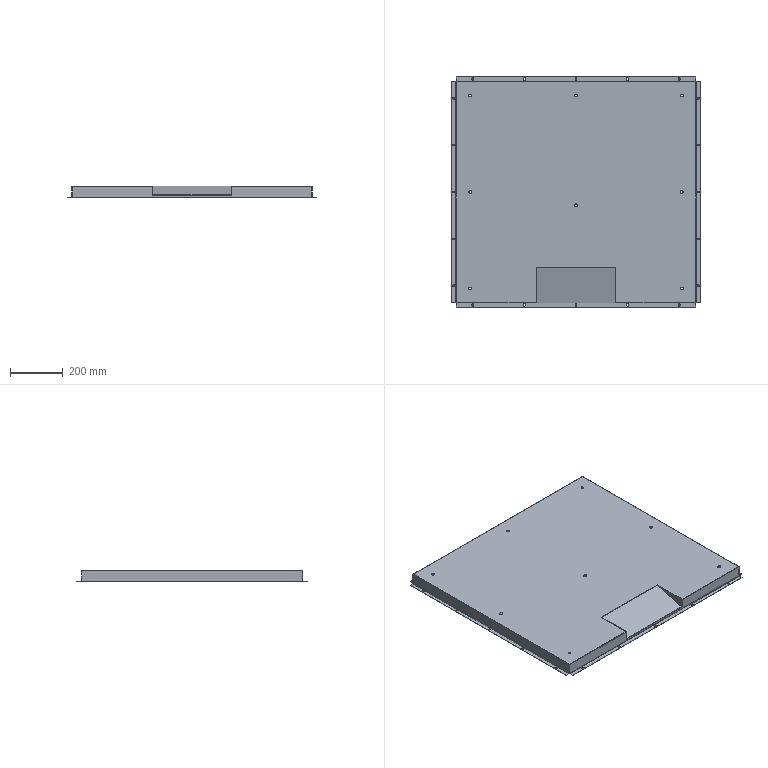Part | 2 solids | 206 faces | box 940 x 870 x 44 mm | volume 956905 mm3 | plane 106 | cylinder 88 | spline 12 | commonest cylinder face diameters 7 x50 11 x16 1 x9 3 x9 0.4 x2 2.4 x2